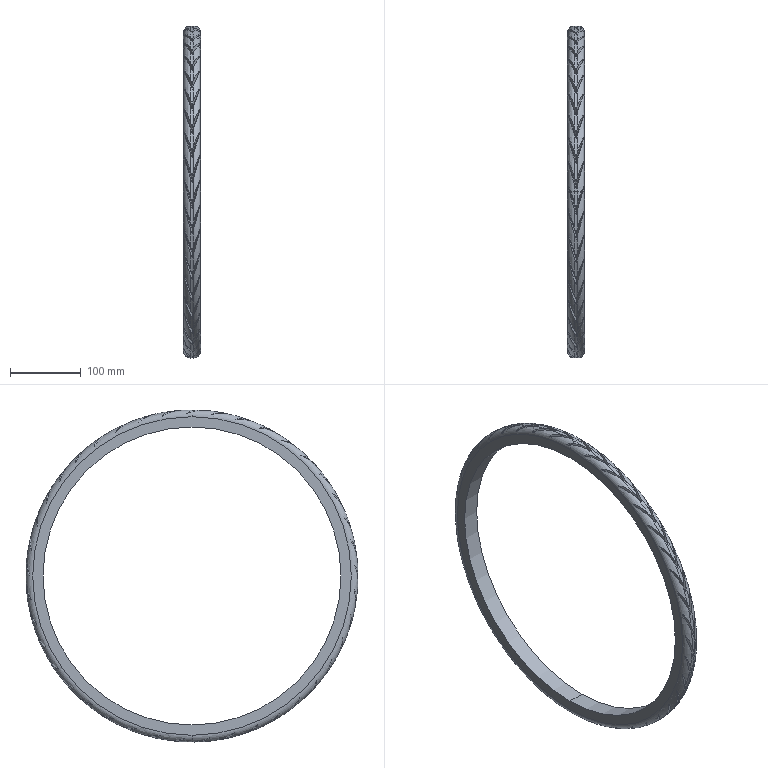Part | STEP file | Royce Quick Tyre | 1 solid | 216 faces | box 24 x 468 x 468 mm | volume 731507 mm3 | spline 164 | cylinder 44 | torus 6 | plane 2 | commonest cylinder face diameters 468 x42 420 x2